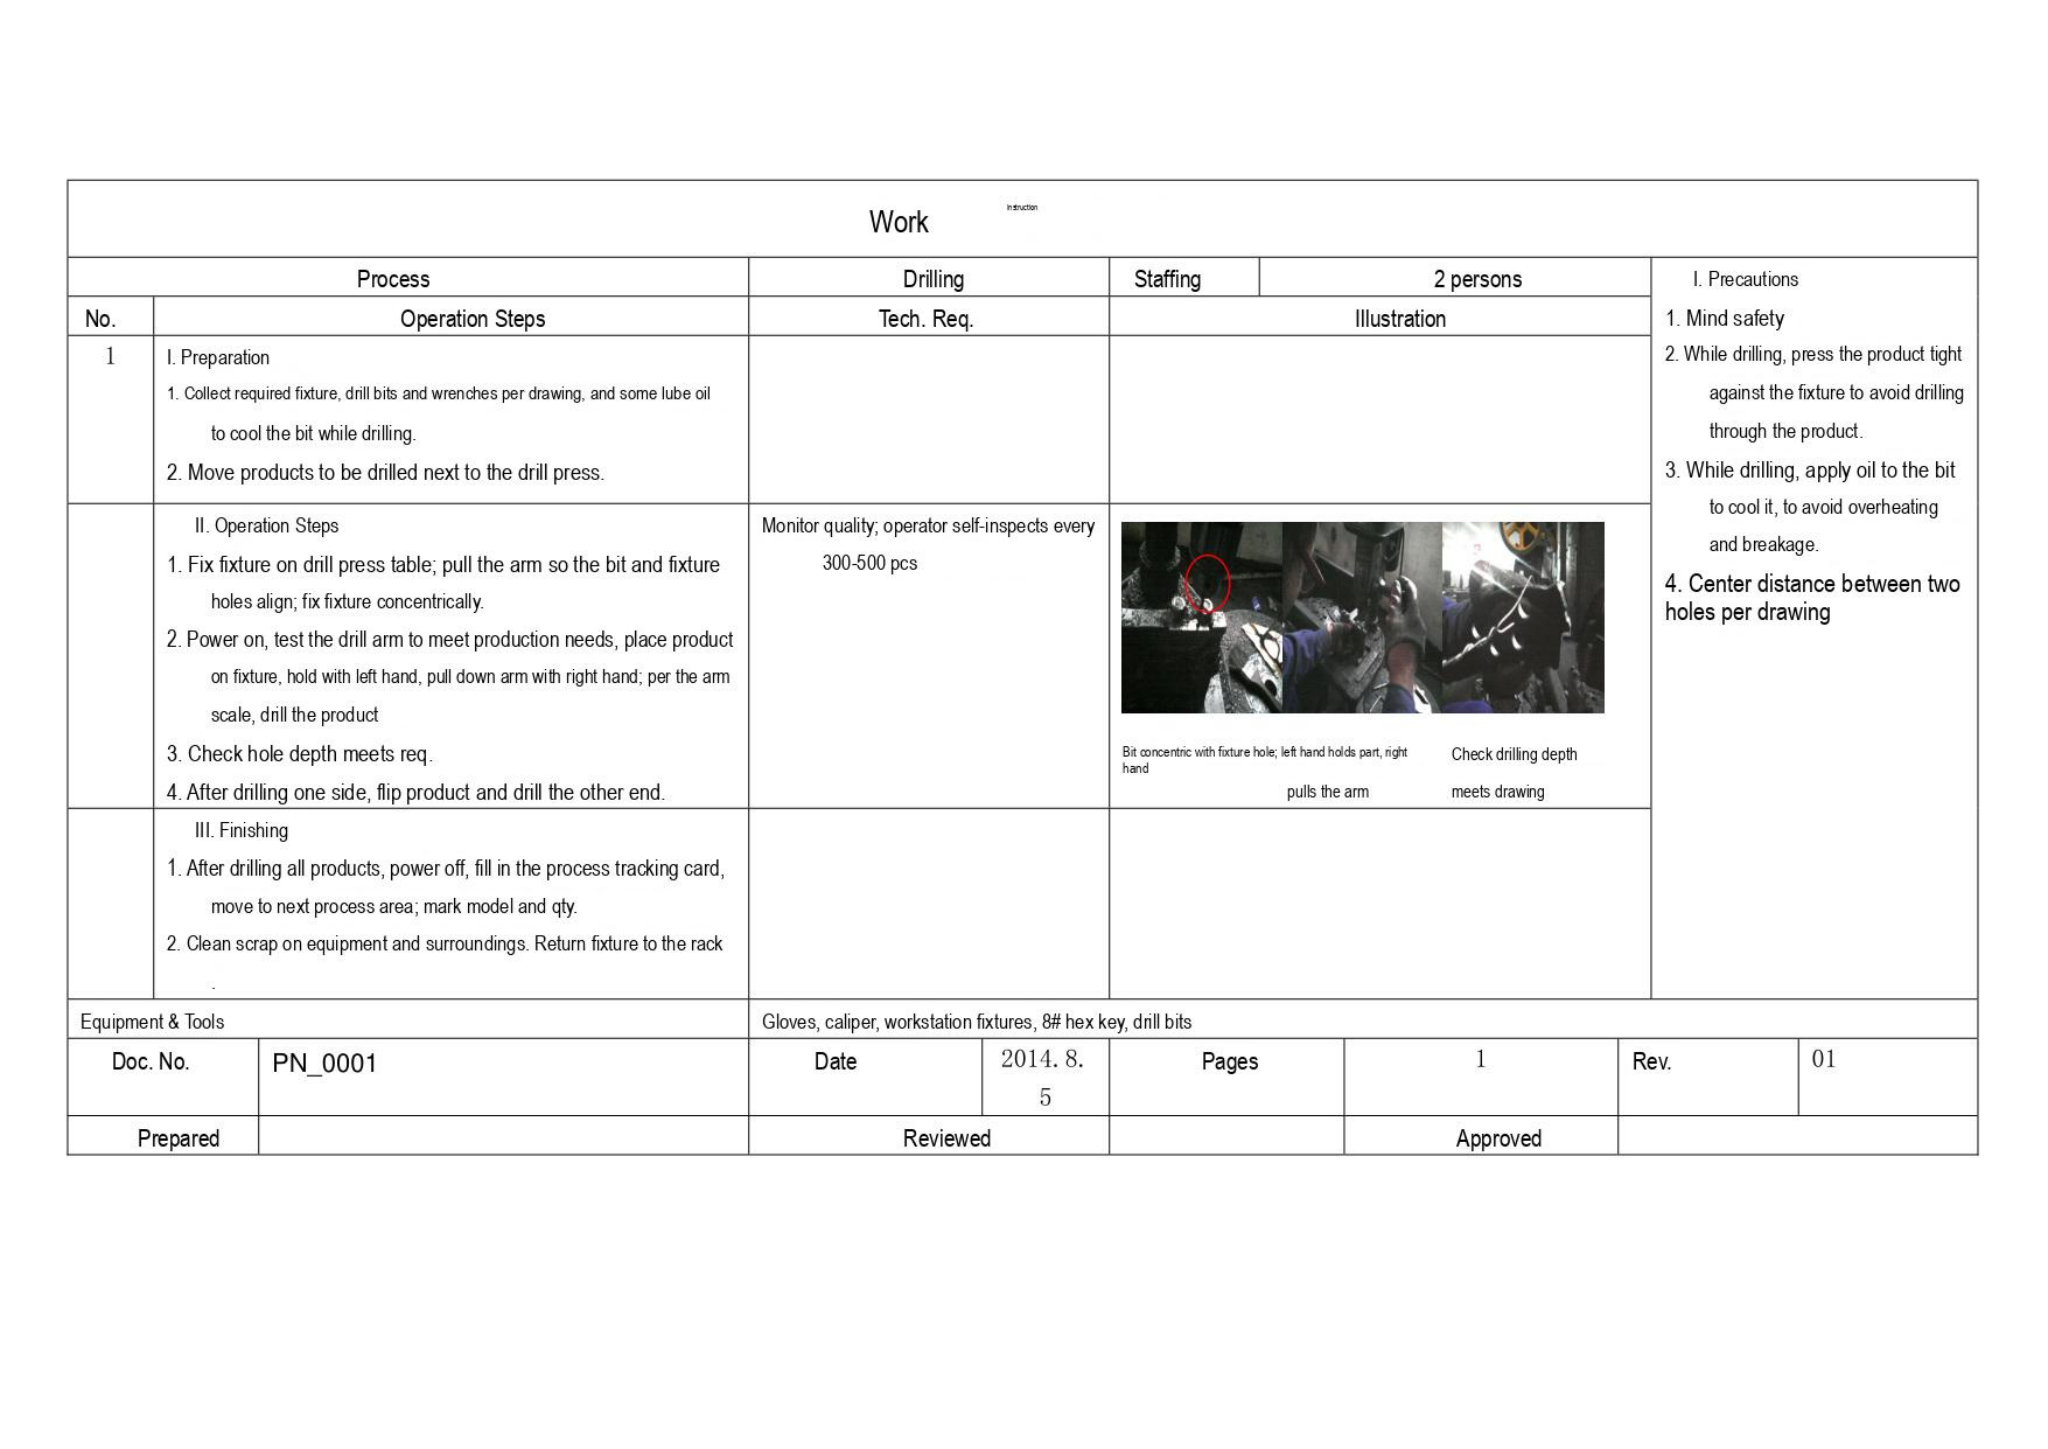Work Instruction

| Process | | Drilling | Staffing | 2 persons | I. Precautions |
|---|---|---|---|---|---|
| **No.** | **Operation Steps** | **Tech. Req.** | **Illustration** | | 1. Mind safety<br>2. While drilling, press the product tight against the fixture to avoid drilling through the product.<br>3. While drilling, apply oil to the bit to cool it, to avoid overheating and breakage.<br>4. Center distance between two holes per drawing |
| 1 | I. Preparation<br>1. Collect required fixture, drill bits and wrenches per drawing, and some lube oil to cool the bit while drilling.<br>2. Move products to be drilled next to the drill press. | | | | |
| | II. Operation Steps<br>1. Fix fixture on drill press table; pull the arm so the bit and fixture holes align; fix fixture concentrically.<br>2. Power on, test the drill arm to meet production needs, place product on fixture, hold with left hand, pull down arm with right hand; per the arm scale, drill the product<br>3. Check hole depth meets req.<br>4. After drilling one side, flip product and drill the other end. | Monitor quality; operator self-inspects every 300-500 pcs | Bit concentric with fixture hole; left hand holds part, right hand pulls the arm<br>Check drilling depth meets drawing | | |
| | III. Finishing<br>1. After drilling all products, power off, fill in the process tracking card, move to next process area; mark model and qty.<br>2. Clean scrap on equipment and surroundings. Return fixture to the rack. | | | | |

| Equipment & Tools | Gloves, caliper, workstation fixtures, 8# hex key, drill bits |
|---|---|

| Doc. No. | PN_0001 | Date | 2014. 8. 5 | Pages | 1 | Rev. | 01 |
|---|---|---|---|---|---|---|---|
| Prepared | | Reviewed | | | Approved | | |